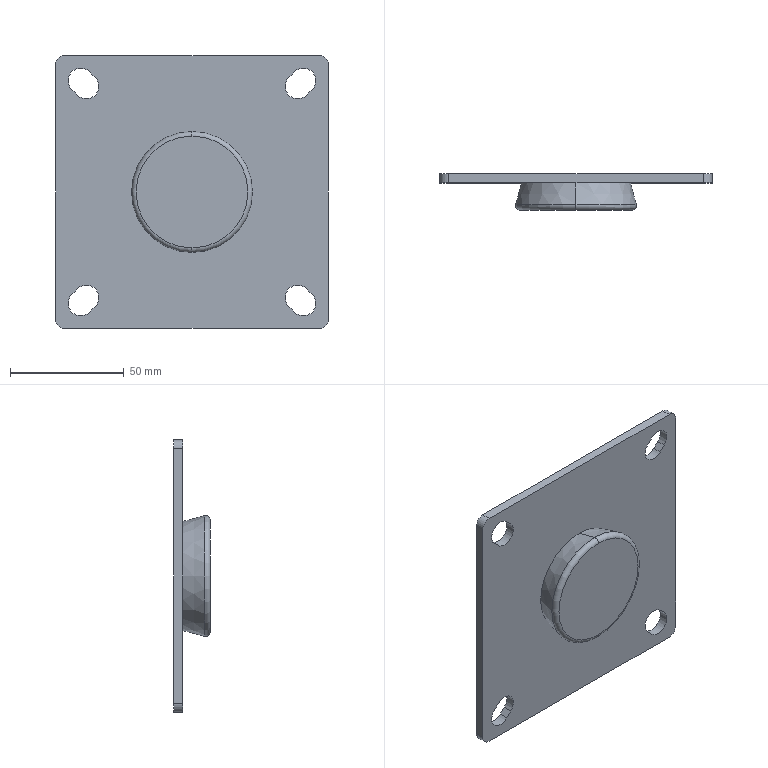Part | STEP file | JAJ-65_plate | 1 solid | 31 faces | box 120 x 16 x 120 mm | volume 79899 mm3 | plane 15 | cylinder 12 | torus 2 | cone 2 | commonest cylinder face diameters 11 x8 8 x4
STEP:
#1=CARTESIAN_POINT('',(0.,-9.482,26.541));
#2=VERTEX_POINT('',#1);
#3=CARTESIAN_POINT('',(0.,-9.482,-26.541));
#4=VERTEX_POINT('',#3);
#5=CARTESIAN_POINT('',(0.,-9.482,0.));
#6=DIRECTION('',(0.,-1.,0.));
#7=DIRECTION('',(0.,0.,-1.));
#8=AXIS2_PLACEMENT_3D('',#5,#6,#7);
#9=CIRCLE('',#8,26.541);
#10=EDGE_CURVE('',#2,#4,#9,.T.);
#11=ORIENTED_EDGE('',*,*,#10,.T.);
#12=CARTESIAN_POINT('',(0.,-12.,-24.609));
#13=VERTEX_POINT('',#12);
#14=CARTESIAN_POINT('',(0.,-10.,-24.609));
#15=DIRECTION('',(-1.,0.,0.));
#16=DIRECTION('',(0.,0.,1.));
#17=AXIS2_PLACEMENT_3D('',#14,#15,#16);
#18=CIRCLE('',#17,2.);
#19=EDGE_CURVE('',#4,#13,#18,.T.);
#20=ORIENTED_EDGE('',*,*,#19,.T.);
#21=CARTESIAN_POINT('',(0.,-12.,24.609));
#22=VERTEX_POINT('',#21);
#23=CARTESIAN_POINT('',(0.,-12.,0.));
#24=DIRECTION('',(0.,-1.,0.));
#25=DIRECTION('',(0.,0.,1.));
#26=AXIS2_PLACEMENT_3D('',#23,#24,#25);
#27=CIRCLE('',#26,24.609);
#28=EDGE_CURVE('',#22,#13,#27,.T.);
#29=ORIENTED_EDGE('',*,*,#28,.F.);
#30=CARTESIAN_POINT('',(0.,-10.,24.609));
#31=DIRECTION('',(1.,0.,0.));
#32=DIRECTION('',(0.,0.,-1.));
#33=AXIS2_PLACEMENT_3D('',#30,#31,#32);
#34=CIRCLE('',#33,2.);
#35=EDGE_CURVE('',#2,#22,#34,.T.);
#36=ORIENTED_EDGE('',*,*,#35,.F.);
#37=EDGE_LOOP('',(#11,#20,#29,#36));
#38=FACE_OUTER_BOUND('',#37,.T.);
#39=CARTESIAN_POINT('',(0.,-10.,0.));
#40=DIRECTION('',(0.,-1.,0.));
#41=DIRECTION('',(0.,0.,1.));
#42=AXIS2_PLACEMENT_3D('',#39,#40,#41);
#43=TOROIDAL_SURFACE('',#42,24.609,2.);
#44=ADVANCED_FACE('',(#38),#43,.T.);
#45=CARTESIAN_POINT('',(0.,0.,24.));
#46=VERTEX_POINT('',#45);
#47=CARTESIAN_POINT('',(0.,0.,-24.));
#48=VERTEX_POINT('',#47);
#49=CARTESIAN_POINT('',(0.,0.,0.));
#50=DIRECTION('',(0.,-1.,0.));
#51=DIRECTION('',(0.,0.,-1.));
#52=AXIS2_PLACEMENT_3D('',#49,#50,#51);
#53=CIRCLE('',#52,24.);
#54=EDGE_CURVE('',#46,#48,#53,.T.);
#55=ORIENTED_EDGE('',*,*,#54,.T.);
#56=CARTESIAN_POINT('',(0.,-9.482,-26.541));
#57=DIRECTION('',(0.,-0.9659,-0.2588));
#58=VECTOR('',#57,1000.);
#59=LINE('',#56,#58);
#60=EDGE_CURVE('',#48,#4,#59,.T.);
#61=ORIENTED_EDGE('',*,*,#60,.T.);
#62=ORIENTED_EDGE('',*,*,#10,.F.);
#63=CARTESIAN_POINT('',(0.,-9.482,26.541));
#64=DIRECTION('',(0.,-0.9659,0.2588));
#65=VECTOR('',#64,1000.);
#66=LINE('',#63,#65);
#67=EDGE_CURVE('',#46,#2,#66,.T.);
#68=ORIENTED_EDGE('',*,*,#67,.F.);
#69=EDGE_LOOP('',(#55,#61,#62,#68));
#70=FACE_OUTER_BOUND('',#69,.T.);
#71=CARTESIAN_POINT('',(0.,-9.482,0.));
#72=DIRECTION('',(0.,-1.,0.));
#73=DIRECTION('',(0.,0.,1.));
#74=AXIS2_PLACEMENT_3D('',#71,#72,#73);
#75=CONICAL_SURFACE('',#74,26.541,0.2618);
#76=ADVANCED_FACE('',(#70),#75,.T.);
#77=CARTESIAN_POINT('',(-60.,0.,-56.));
#78=VERTEX_POINT('',#77);
#79=CARTESIAN_POINT('',(-60.,0.,56.));
#80=VERTEX_POINT('',#79);
#81=CARTESIAN_POINT('',(-60.,0.,-56.));
#82=DIRECTION('',(0.,0.,1.));
#83=VECTOR('',#82,1000.);
#84=LINE('',#81,#83);
#85=EDGE_CURVE('',#78,#80,#84,.T.);
#86=ORIENTED_EDGE('',*,*,#85,.T.);
#87=CARTESIAN_POINT('',(-60.,4.,56.));
#88=VERTEX_POINT('',#87);
#89=CARTESIAN_POINT('',(-60.,0.,56.));
#90=DIRECTION('',(0.,-1.,0.));
#91=VECTOR('',#90,1000.);
#92=LINE('',#89,#91);
#93=EDGE_CURVE('',#88,#80,#92,.T.);
#94=ORIENTED_EDGE('',*,*,#93,.F.);
#95=CARTESIAN_POINT('',(-60.,4.,-56.));
#96=VERTEX_POINT('',#95);
#97=CARTESIAN_POINT('',(-60.,4.,56.));
#98=DIRECTION('',(0.,0.,1.));
#99=VECTOR('',#98,1000.);
#100=LINE('',#97,#99);
#101=EDGE_CURVE('',#96,#88,#100,.T.);
#102=ORIENTED_EDGE('',*,*,#101,.F.);
#103=CARTESIAN_POINT('',(-60.,4.,-56.));
#104=DIRECTION('',(0.,-1.,0.));
#105=VECTOR('',#104,1000.);
#106=LINE('',#103,#105);
#107=EDGE_CURVE('',#96,#78,#106,.T.);
#108=ORIENTED_EDGE('',*,*,#107,.T.);
#109=EDGE_LOOP('',(#86,#94,#102,#108));
#110=FACE_OUTER_BOUND('',#109,.T.);
#111=CARTESIAN_POINT('',(-60.,0.,56.));
#112=DIRECTION('',(-1.,0.,0.));
#113=DIRECTION('',(0.,1.,0.));
#114=AXIS2_PLACEMENT_3D('',#111,#112,#113);
#115=PLANE('',#114);
#116=ADVANCED_FACE('',(#110),#115,.T.);
#117=CARTESIAN_POINT('',(-56.,0.,60.));
#118=VERTEX_POINT('',#117);
#119=CARTESIAN_POINT('',(-56.,0.,56.));
#120=DIRECTION('',(0.,1.,0.));
#121=DIRECTION('',(-1.,0.,0.));
#122=AXIS2_PLACEMENT_3D('',#119,#120,#121);
#123=CIRCLE('',#122,4.);
#124=EDGE_CURVE('',#80,#118,#123,.T.);
#125=ORIENTED_EDGE('',*,*,#124,.T.);
#126=CARTESIAN_POINT('',(-56.,4.,60.));
#127=VERTEX_POINT('',#126);
#128=CARTESIAN_POINT('',(-56.,0.,60.));
#129=DIRECTION('',(0.,-1.,0.));
#130=VECTOR('',#129,1000.);
#131=LINE('',#128,#130);
#132=EDGE_CURVE('',#127,#118,#131,.T.);
#133=ORIENTED_EDGE('',*,*,#132,.F.);
#134=CARTESIAN_POINT('',(-56.,4.,56.));
#135=DIRECTION('',(0.,1.,0.));
#136=DIRECTION('',(0.,0.,1.));
#137=AXIS2_PLACEMENT_3D('',#134,#135,#136);
#138=CIRCLE('',#137,4.);
#139=EDGE_CURVE('',#88,#127,#138,.T.);
#140=ORIENTED_EDGE('',*,*,#139,.F.);
#141=ORIENTED_EDGE('',*,*,#93,.T.);
#142=EDGE_LOOP('',(#125,#133,#140,#141));
#143=FACE_OUTER_BOUND('',#142,.T.);
#144=CARTESIAN_POINT('',(-56.,4.,56.));
#145=DIRECTION('',(0.,-1.,0.));
#146=DIRECTION('',(0.,0.,1.));
#147=AXIS2_PLACEMENT_3D('',#144,#145,#146);
#148=CYLINDRICAL_SURFACE('',#147,4.);
#149=ADVANCED_FACE('',(#143),#148,.T.);
#150=CARTESIAN_POINT('',(56.,0.,60.));
#151=VERTEX_POINT('',#150);
#152=CARTESIAN_POINT('',(-56.,0.,60.));
#153=DIRECTION('',(1.,0.,0.));
#154=VECTOR('',#153,1000.);
#155=LINE('',#152,#154);
#156=EDGE_CURVE('',#118,#151,#155,.T.);
#157=ORIENTED_EDGE('',*,*,#156,.T.);
#158=CARTESIAN_POINT('',(56.,4.,60.));
#159=VERTEX_POINT('',#158);
#160=CARTESIAN_POINT('',(56.,0.,60.));
#161=DIRECTION('',(0.,-1.,0.));
#162=VECTOR('',#161,1000.);
#163=LINE('',#160,#162);
#164=EDGE_CURVE('',#159,#151,#163,.T.);
#165=ORIENTED_EDGE('',*,*,#164,.F.);
#166=CARTESIAN_POINT('',(56.,4.,60.));
#167=DIRECTION('',(1.,0.,0.));
#168=VECTOR('',#167,1000.);
#169=LINE('',#166,#168);
#170=EDGE_CURVE('',#127,#159,#169,.T.);
#171=ORIENTED_EDGE('',*,*,#170,.F.);
#172=ORIENTED_EDGE('',*,*,#132,.T.);
#173=EDGE_LOOP('',(#157,#165,#171,#172));
#174=FACE_OUTER_BOUND('',#173,.T.);
#175=CARTESIAN_POINT('',(56.,0.,60.));
#176=DIRECTION('',(0.,0.,1.));
#177=DIRECTION('',(0.,1.,0.));
#178=AXIS2_PLACEMENT_3D('',#175,#176,#177);
#179=PLANE('',#178);
#180=ADVANCED_FACE('',(#174),#179,.T.);
#181=CARTESIAN_POINT('',(60.,0.,56.));
#182=VERTEX_POINT('',#181);
#183=CARTESIAN_POINT('',(56.,0.,56.));
#184=DIRECTION('',(0.,1.,0.));
#185=DIRECTION('',(0.,0.,1.));
#186=AXIS2_PLACEMENT_3D('',#183,#184,#185);
#187=CIRCLE('',#186,4.);
#188=EDGE_CURVE('',#151,#182,#187,.T.);
#189=ORIENTED_EDGE('',*,*,#188,.T.);
#190=CARTESIAN_POINT('',(60.,4.,56.));
#191=VERTEX_POINT('',#190);
#192=CARTESIAN_POINT('',(60.,0.,56.));
#193=DIRECTION('',(0.,-1.,0.));
#194=VECTOR('',#193,1000.);
#195=LINE('',#192,#194);
#196=EDGE_CURVE('',#191,#182,#195,.T.);
#197=ORIENTED_EDGE('',*,*,#196,.F.);
#198=CARTESIAN_POINT('',(56.,4.,56.));
#199=DIRECTION('',(0.,1.,0.));
#200=DIRECTION('',(1.,0.,0.));
#201=AXIS2_PLACEMENT_3D('',#198,#199,#200);
#202=CIRCLE('',#201,4.);
#203=EDGE_CURVE('',#159,#191,#202,.T.);
#204=ORIENTED_EDGE('',*,*,#203,.F.);
#205=ORIENTED_EDGE('',*,*,#164,.T.);
#206=EDGE_LOOP('',(#189,#197,#204,#205));
#207=FACE_OUTER_BOUND('',#206,.T.);
#208=CARTESIAN_POINT('',(56.,4.,56.));
#209=DIRECTION('',(0.,-1.,0.));
#210=DIRECTION('',(1.,0.,0.));
#211=AXIS2_PLACEMENT_3D('',#208,#209,#210);
#212=CYLINDRICAL_SURFACE('',#211,4.);
#213=ADVANCED_FACE('',(#207),#212,.T.);
#214=CARTESIAN_POINT('',(60.,0.,-56.));
#215=VERTEX_POINT('',#214);
#216=CARTESIAN_POINT('',(60.,0.,56.));
#217=DIRECTION('',(0.,0.,-1.));
#218=VECTOR('',#217,1000.);
#219=LINE('',#216,#218);
#220=EDGE_CURVE('',#182,#215,#219,.T.);
#221=ORIENTED_EDGE('',*,*,#220,.T.);
#222=CARTESIAN_POINT('',(60.,4.,-56.));
#223=VERTEX_POINT('',#222);
#224=CARTESIAN_POINT('',(60.,0.,-56.));
#225=DIRECTION('',(0.,-1.,0.));
#226=VECTOR('',#225,1000.);
#227=LINE('',#224,#226);
#228=EDGE_CURVE('',#223,#215,#227,.T.);
#229=ORIENTED_EDGE('',*,*,#228,.F.);
#230=CARTESIAN_POINT('',(60.,4.,-56.));
#231=DIRECTION('',(0.,0.,-1.));
#232=VECTOR('',#231,1000.);
#233=LINE('',#230,#232);
#234=EDGE_CURVE('',#191,#223,#233,.T.);
#235=ORIENTED_EDGE('',*,*,#234,.F.);
#236=ORIENTED_EDGE('',*,*,#196,.T.);
#237=EDGE_LOOP('',(#221,#229,#235,#236));
#238=FACE_OUTER_BOUND('',#237,.T.);
#239=CARTESIAN_POINT('',(60.,0.,-56.));
#240=DIRECTION('',(1.,0.,0.));
#241=DIRECTION('',(0.,1.,0.));
#242=AXIS2_PLACEMENT_3D('',#239,#240,#241);
#243=PLANE('',#242);
#244=ADVANCED_FACE('',(#238),#243,.T.);
#245=CARTESIAN_POINT('',(56.,0.,-60.));
#246=VERTEX_POINT('',#245);
#247=CARTESIAN_POINT('',(56.,0.,-56.));
#248=DIRECTION('',(0.,1.,0.));
#249=DIRECTION('',(1.,0.,0.));
#250=AXIS2_PLACEMENT_3D('',#247,#248,#249);
#251=CIRCLE('',#250,4.);
#252=EDGE_CURVE('',#215,#246,#251,.T.);
#253=ORIENTED_EDGE('',*,*,#252,.T.);
#254=CARTESIAN_POINT('',(56.,4.,-60.));
#255=VERTEX_POINT('',#254);
#256=CARTESIAN_POINT('',(56.,0.,-60.));
#257=DIRECTION('',(0.,-1.,0.));
#258=VECTOR('',#257,1000.);
#259=LINE('',#256,#258);
#260=EDGE_CURVE('',#255,#246,#259,.T.);
#261=ORIENTED_EDGE('',*,*,#260,.F.);
#262=CARTESIAN_POINT('',(56.,4.,-56.));
#263=DIRECTION('',(0.,1.,0.));
#264=DIRECTION('',(0.,0.,-1.));
#265=AXIS2_PLACEMENT_3D('',#262,#263,#264);
#266=CIRCLE('',#265,4.);
#267=EDGE_CURVE('',#223,#255,#266,.T.);
#268=ORIENTED_EDGE('',*,*,#267,.F.);
#269=ORIENTED_EDGE('',*,*,#228,.T.);
#270=EDGE_LOOP('',(#253,#261,#268,#269));
#271=FACE_OUTER_BOUND('',#270,.T.);
#272=CARTESIAN_POINT('',(56.,4.,-56.));
#273=DIRECTION('',(0.,-1.,0.));
#274=DIRECTION('',(0.,0.,-1.));
#275=AXIS2_PLACEMENT_3D('',#272,#273,#274);
#276=CYLINDRICAL_SURFACE('',#275,4.);
#277=ADVANCED_FACE('',(#271),#276,.T.);
#278=CARTESIAN_POINT('',(-56.,0.,-60.));
#279=VERTEX_POINT('',#278);
#280=CARTESIAN_POINT('',(56.,0.,-60.));
#281=DIRECTION('',(-1.,0.,0.));
#282=VECTOR('',#281,1000.);
#283=LINE('',#280,#282);
#284=EDGE_CURVE('',#246,#279,#283,.T.);
#285=ORIENTED_EDGE('',*,*,#284,.T.);
#286=CARTESIAN_POINT('',(-56.,4.,-60.));
#287=VERTEX_POINT('',#286);
#288=CARTESIAN_POINT('',(-56.,0.,-60.));
#289=DIRECTION('',(0.,-1.,0.));
#290=VECTOR('',#289,1000.);
#291=LINE('',#288,#290);
#292=EDGE_CURVE('',#287,#279,#291,.T.);
#293=ORIENTED_EDGE('',*,*,#292,.F.);
#294=CARTESIAN_POINT('',(-56.,4.,-60.));
#295=DIRECTION('',(-1.,0.,0.));
#296=VECTOR('',#295,1000.);
#297=LINE('',#294,#296);
#298=EDGE_CURVE('',#255,#287,#297,.T.);
#299=ORIENTED_EDGE('',*,*,#298,.F.);
#300=ORIENTED_EDGE('',*,*,#260,.T.);
#301=EDGE_LOOP('',(#285,#293,#299,#300));
#302=FACE_OUTER_BOUND('',#301,.T.);
#303=CARTESIAN_POINT('',(-56.,0.,-60.));
#304=DIRECTION('',(0.,0.,-1.));
#305=DIRECTION('',(0.,1.,0.));
#306=AXIS2_PLACEMENT_3D('',#303,#304,#305);
#307=PLANE('',#306);
#308=ADVANCED_FACE('',(#302),#307,.T.);
#309=CARTESIAN_POINT('',(45.111,0.,-52.889));
#310=VERTEX_POINT('',#309);
#311=CARTESIAN_POINT('',(42.611,0.,-50.389));
#312=VERTEX_POINT('',#311);
#313=CARTESIAN_POINT('',(42.611,0.,-50.389));
#314=DIRECTION('',(-0.7071,0.,0.7071));
#315=VECTOR('',#314,1000.);
#316=LINE('',#313,#315);
#317=EDGE_CURVE('',#310,#312,#316,.T.);
#318=ORIENTED_EDGE('',*,*,#317,.F.);
#319=CARTESIAN_POINT('',(45.111,4.,-52.889));
#320=VERTEX_POINT('',#319);
#321=CARTESIAN_POINT('',(45.111,0.,-52.889));
#322=DIRECTION('',(0.,-1.,0.));
#323=VECTOR('',#322,1000.);
#324=LINE('',#321,#323);
#325=EDGE_CURVE('',#320,#310,#324,.T.);
#326=ORIENTED_EDGE('',*,*,#325,.F.);
#327=CARTESIAN_POINT('',(42.611,4.,-50.389));
#328=VERTEX_POINT('',#327);
#329=CARTESIAN_POINT('',(45.111,4.,-52.889));
#330=DIRECTION('',(-0.7071,0.,0.7071));
#331=VECTOR('',#330,1000.);
#332=LINE('',#329,#331);
#333=EDGE_CURVE('',#320,#328,#332,.T.);
#334=ORIENTED_EDGE('',*,*,#333,.T.);
#335=CARTESIAN_POINT('',(42.611,4.,-50.389));
#336=DIRECTION('',(0.,-1.,0.));
#337=VECTOR('',#336,1000.);
#338=LINE('',#335,#337);
#339=EDGE_CURVE('',#328,#312,#338,.T.);
#340=ORIENTED_EDGE('',*,*,#339,.T.);
#341=EDGE_LOOP('',(#318,#326,#334,#340));
#342=FACE_OUTER_BOUND('',#341,.T.);
#343=CARTESIAN_POINT('',(42.611,0.,-50.389));
#344=DIRECTION('',(0.7071,0.,0.7071));
#345=DIRECTION('',(0.7071,0.,-0.7071));
#346=AXIS2_PLACEMENT_3D('',#343,#344,#345);
#347=PLANE('',#346);
#348=ADVANCED_FACE('',(#342),#347,.T.);
#349=CARTESIAN_POINT('',(52.889,0.,-45.111));
#350=VERTEX_POINT('',#349);
#351=CARTESIAN_POINT('',(49.,0.,-49.));
#352=DIRECTION('',(0.,1.,0.));
#353=DIRECTION('',(-0.7071,0.,-0.7071));
#354=AXIS2_PLACEMENT_3D('',#351,#352,#353);
#355=CIRCLE('',#354,5.5);
#356=EDGE_CURVE('',#350,#310,#355,.T.);
#357=ORIENTED_EDGE('',*,*,#356,.F.);
#358=CARTESIAN_POINT('',(52.889,4.,-45.111));
#359=VERTEX_POINT('',#358);
#360=CARTESIAN_POINT('',(52.889,0.,-45.111));
#361=DIRECTION('',(0.,-1.,0.));
#362=VECTOR('',#361,1000.);
#363=LINE('',#360,#362);
#364=EDGE_CURVE('',#359,#350,#363,.T.);
#365=ORIENTED_EDGE('',*,*,#364,.F.);
#366=CARTESIAN_POINT('',(49.,4.,-49.));
#367=DIRECTION('',(0.,1.,0.));
#368=DIRECTION('',(0.7071,0.,0.7071));
#369=AXIS2_PLACEMENT_3D('',#366,#367,#368);
#370=CIRCLE('',#369,5.5);
#371=EDGE_CURVE('',#359,#320,#370,.T.);
#372=ORIENTED_EDGE('',*,*,#371,.T.);
#373=ORIENTED_EDGE('',*,*,#325,.T.);
#374=EDGE_LOOP('',(#357,#365,#372,#373));
#375=FACE_OUTER_BOUND('',#374,.T.);
#376=CARTESIAN_POINT('',(49.,4.,-49.));
#377=DIRECTION('',(0.,-1.,0.));
#378=DIRECTION('',(-0.7071,0.,-0.7071));
#379=AXIS2_PLACEMENT_3D('',#376,#377,#378);
#380=CYLINDRICAL_SURFACE('',#379,5.5);
#381=ADVANCED_FACE('',(#375),#380,.F.);
#382=CARTESIAN_POINT('',(50.389,0.,-42.611));
#383=VERTEX_POINT('',#382);
#384=CARTESIAN_POINT('',(52.889,0.,-45.111));
#385=DIRECTION('',(0.7071,0.,-0.7071));
#386=VECTOR('',#385,1000.);
#387=LINE('',#384,#386);
#388=EDGE_CURVE('',#383,#350,#387,.T.);
#389=ORIENTED_EDGE('',*,*,#388,.F.);
#390=CARTESIAN_POINT('',(50.389,4.,-42.611));
#391=VERTEX_POINT('',#390);
#392=CARTESIAN_POINT('',(50.389,0.,-42.611));
#393=DIRECTION('',(0.,-1.,0.));
#394=VECTOR('',#393,1000.);
#395=LINE('',#392,#394);
#396=EDGE_CURVE('',#391,#383,#395,.T.);
#397=ORIENTED_EDGE('',*,*,#396,.F.);
#398=CARTESIAN_POINT('',(50.389,4.,-42.611));
#399=DIRECTION('',(0.7071,0.,-0.7071));
#400=VECTOR('',#399,1000.);
#401=LINE('',#398,#400);
#402=EDGE_CURVE('',#391,#359,#401,.T.);
#403=ORIENTED_EDGE('',*,*,#402,.T.);
#404=ORIENTED_EDGE('',*,*,#364,.T.);
#405=EDGE_LOOP('',(#389,#397,#403,#404));
#406=FACE_OUTER_BOUND('',#405,.T.);
#407=CARTESIAN_POINT('',(52.889,0.,-45.111));
#408=DIRECTION('',(-0.7071,0.,-0.7071));
#409=DIRECTION('',(-0.7071,0.,0.7071));
#410=AXIS2_PLACEMENT_3D('',#407,#408,#409);
#411=PLANE('',#410);
#412=ADVANCED_FACE('',(#406),#411,.T.);
#413=CARTESIAN_POINT('',(52.889,0.,45.111));
#414=VERTEX_POINT('',#413);
#415=CARTESIAN_POINT('',(50.389,0.,42.611));
#416=VERTEX_POINT('',#415);
#417=CARTESIAN_POINT('',(50.389,0.,42.611));
#418=DIRECTION('',(-0.7071,0.,-0.7071));
#419=VECTOR('',#418,1000.);
#420=LINE('',#417,#419);
#421=EDGE_CURVE('',#414,#416,#420,.T.);
#422=ORIENTED_EDGE('',*,*,#421,.F.);
#423=CARTESIAN_POINT('',(52.889,4.,45.111));
#424=VERTEX_POINT('',#423);
#425=CARTESIAN_POINT('',(52.889,0.,45.111));
#426=DIRECTION('',(0.,-1.,0.));
#427=VECTOR('',#426,1000.);
#428=LINE('',#425,#427);
#429=EDGE_CURVE('',#424,#414,#428,.T.);
#430=ORIENTED_EDGE('',*,*,#429,.F.);
#431=CARTESIAN_POINT('',(50.389,4.,42.611));
#432=VERTEX_POINT('',#431);
#433=CARTESIAN_POINT('',(52.889,4.,45.111));
#434=DIRECTION('',(-0.7071,0.,-0.7071));
#435=VECTOR('',#434,1000.);
#436=LINE('',#433,#435);
#437=EDGE_CURVE('',#424,#432,#436,.T.);
#438=ORIENTED_EDGE('',*,*,#437,.T.);
#439=CARTESIAN_POINT('',(50.389,4.,42.611));
#440=DIRECTION('',(0.,-1.,0.));
#441=VECTOR('',#440,1000.);
#442=LINE('',#439,#441);
#443=EDGE_CURVE('',#432,#416,#442,.T.);
#444=ORIENTED_EDGE('',*,*,#443,.T.);
#445=EDGE_LOOP('',(#422,#430,#438,#444));
#446=FACE_OUTER_BOUND('',#445,.T.);
#447=CARTESIAN_POINT('',(50.389,0.,42.611));
#448=DIRECTION('',(-0.7071,0.,0.7071));
#449=DIRECTION('',(0.7071,0.,0.7071));
#450=AXIS2_PLACEMENT_3D('',#447,#448,#449);
#451=PLANE('',#450);
#452=ADVANCED_FACE('',(#446),#451,.T.);
#453=CARTESIAN_POINT('',(45.111,0.,52.889));
#454=VERTEX_POINT('',#453);
#455=CARTESIAN_POINT('',(49.,0.,49.));
#456=DIRECTION('',(0.,1.,0.));
#457=DIRECTION('',(0.7071,0.,-0.7071));
#458=AXIS2_PLACEMENT_3D('',#455,#456,#457);
#459=CIRCLE('',#458,5.5);
#460=EDGE_CURVE('',#454,#414,#459,.T.);
#461=ORIENTED_EDGE('',*,*,#460,.F.);
#462=CARTESIAN_POINT('',(45.111,4.,52.889));
#463=VERTEX_POINT('',#462);
#464=CARTESIAN_POINT('',(45.111,0.,52.889));
#465=DIRECTION('',(0.,-1.,0.));
#466=VECTOR('',#465,1000.);
#467=LINE('',#464,#466);
#468=EDGE_CURVE('',#463,#454,#467,.T.);
#469=ORIENTED_EDGE('',*,*,#468,.F.);
#470=CARTESIAN_POINT('',(49.,4.,49.));
#471=DIRECTION('',(0.,1.,0.));
#472=DIRECTION('',(-0.7071,0.,0.7071));
#473=AXIS2_PLACEMENT_3D('',#470,#471,#472);
#474=CIRCLE('',#473,5.5);
#475=EDGE_CURVE('',#463,#424,#474,.T.);
#476=ORIENTED_EDGE('',*,*,#475,.T.);
#477=ORIENTED_EDGE('',*,*,#429,.T.);
#478=EDGE_LOOP('',(#461,#469,#476,#477));
#479=FACE_OUTER_BOUND('',#478,.T.);
#480=CARTESIAN_POINT('',(49.,4.,49.));
#481=DIRECTION('',(0.,-1.,0.));
#482=DIRECTION('',(0.7071,0.,-0.7071));
#483=AXIS2_PLACEMENT_3D('',#480,#481,#482);
#484=CYLINDRICAL_SURFACE('',#483,5.5);
#485=ADVANCED_FACE('',(#479),#484,.F.);
#486=CARTESIAN_POINT('',(42.611,0.,50.389));
#487=VERTEX_POINT('',#486);
#488=CARTESIAN_POINT('',(45.111,0.,52.889));
#489=DIRECTION('',(0.7071,0.,0.7071));
#490=VECTOR('',#489,1000.);
#491=LINE('',#488,#490);
#492=EDGE_CURVE('',#487,#454,#491,.T.);
#493=ORIENTED_EDGE('',*,*,#492,.F.);
#494=CARTESIAN_POINT('',(42.611,4.,50.389));
#495=VERTEX_POINT('',#494);
#496=CARTESIAN_POINT('',(42.611,0.,50.389));
#497=DIRECTION('',(0.,-1.,0.));
#498=VECTOR('',#497,1000.);
#499=LINE('',#496,#498);
#500=EDGE_CURVE('',#495,#487,#499,.T.);
#501=ORIENTED_EDGE('',*,*,#500,.F.);
#502=CARTESIAN_POINT('',(42.611,4.,50.389));
#503=DIRECTION('',(0.7071,0.,0.7071));
#504=VECTOR('',#503,1000.);
#505=LINE('',#502,#504);
#506=EDGE_CURVE('',#495,#463,#505,.T.);
#507=ORIENTED_EDGE('',*,*,#506,.T.);
#508=ORIENTED_EDGE('',*,*,#468,.T.);
#509=EDGE_LOOP('',(#493,#501,#507,#508));
#510=FACE_OUTER_BOUND('',#509,.T.);
#511=CARTESIAN_POINT('',(45.111,0.,52.889));
#512=DIRECTION('',(0.7071,0.,-0.7071));
#513=DIRECTION('',(-0.7071,0.,-0.7071));
#514=AXIS2_PLACEMENT_3D('',#511,#512,#513);
#515=PLANE('',#514);
#516=ADVANCED_FACE('',(#510),#515,.T.);
#517=CARTESIAN_POINT('',(-42.611,0.,-50.389));
#518=VERTEX_POINT('',#517);
#519=CARTESIAN_POINT('',(-45.111,0.,-52.889));
#520=VERTEX_POINT('',#519);
#521=CARTESIAN_POINT('',(-45.111,0.,-52.889));
#522=DIRECTION('',(-0.7071,0.,-0.7071));
#523=VECTOR('',#522,1000.);
#524=LINE('',#521,#523);
#525=EDGE_CURVE('',#518,#520,#524,.T.);
#526=ORIENTED_EDGE('',*,*,#525,.F.);
#527=CARTESIAN_POINT('',(-42.611,4.,-50.389));
#528=VERTEX_POINT('',#527);
#529=CARTESIAN_POINT('',(-42.611,0.,-50.389));
#530=DIRECTION('',(0.,-1.,0.));
#531=VECTOR('',#530,1000.);
#532=LINE('',#529,#531);
#533=EDGE_CURVE('',#528,#518,#532,.T.);
#534=ORIENTED_EDGE('',*,*,#533,.F.);
#535=CARTESIAN_POINT('',(-45.111,4.,-52.889));
#536=VERTEX_POINT('',#535);
#537=CARTESIAN_POINT('',(-42.611,4.,-50.389));
#538=DIRECTION('',(-0.7071,0.,-0.7071));
#539=VECTOR('',#538,1000.);
#540=LINE('',#537,#539);
#541=EDGE_CURVE('',#528,#536,#540,.T.);
#542=ORIENTED_EDGE('',*,*,#541,.T.);
#543=CARTESIAN_POINT('',(-45.111,4.,-52.889));
#544=DIRECTION('',(0.,-1.,0.));
#545=VECTOR('',#544,1000.);
#546=LINE('',#543,#545);
#547=EDGE_CURVE('',#536,#520,#546,.T.);
#548=ORIENTED_EDGE('',*,*,#547,.T.);
#549=EDGE_LOOP('',(#526,#534,#542,#548));
#550=FACE_OUTER_BOUND('',#549,.T.);
#551=CARTESIAN_POINT('',(-45.111,0.,-52.889));
#552=DIRECTION('',(-0.7071,0.,0.7071));
#553=DIRECTION('',(0.7071,0.,0.7071));
#554=AXIS2_PLACEMENT_3D('',#551,#552,#553);
#555=PLANE('',#554);
#556=ADVANCED_FACE('',(#550),#555,.T.);
#557=CARTESIAN_POINT('',(-50.389,0.,-42.611));
#558=VERTEX_POINT('',#557);
#559=CARTESIAN_POINT('',(-46.5,0.,-46.5));
#560=DIRECTION('',(0.,1.,0.));
#561=DIRECTION('',(0.7071,0.,-0.7071));
#562=AXIS2_PLACEMENT_3D('',#559,#560,#561);
#563=CIRCLE('',#562,5.5);
#564=EDGE_CURVE('',#558,#518,#563,.T.);
#565=ORIENTED_EDGE('',*,*,#564,.F.);
#566=CARTESIAN_POINT('',(-50.389,4.,-42.611));
#567=VERTEX_POINT('',#566);
#568=CARTESIAN_POINT('',(-50.389,0.,-42.611));
#569=DIRECTION('',(0.,-1.,0.));
#570=VECTOR('',#569,1000.);
#571=LINE('',#568,#570);
#572=EDGE_CURVE('',#567,#558,#571,.T.);
#573=ORIENTED_EDGE('',*,*,#572,.F.);
#574=CARTESIAN_POINT('',(-46.5,4.,-46.5));
#575=DIRECTION('',(0.,1.,0.));
#576=DIRECTION('',(-0.7071,0.,0.7071));
#577=AXIS2_PLACEMENT_3D('',#574,#575,#576);
#578=CIRCLE('',#577,5.5);
#579=EDGE_CURVE('',#567,#528,#578,.T.);
#580=ORIENTED_EDGE('',*,*,#579,.T.);
#581=ORIENTED_EDGE('',*,*,#533,.T.);
#582=EDGE_LOOP('',(#565,#573,#580,#581));
#583=FACE_OUTER_BOUND('',#582,.T.);
#584=CARTESIAN_POINT('',(-46.5,4.,-46.5));
#585=DIRECTION('',(0.,-1.,0.));
#586=DIRECTION('',(0.7071,0.,-0.7071));
#587=AXIS2_PLACEMENT_3D('',#584,#585,#586);
#588=CYLINDRICAL_SURFACE('',#587,5.5);
#589=ADVANCED_FACE('',(#583),#588,.F.);
#590=CARTESIAN_POINT('',(-52.889,0.,-45.111));
#591=VERTEX_POINT('',#590);
#592=CARTESIAN_POINT('',(-50.389,0.,-42.611));
#593=DIRECTION('',(0.7071,0.,0.7071));
#594=VECTOR('',#593,1000.);
#595=LINE('',#592,#594);
#596=EDGE_CURVE('',#591,#558,#595,.T.);
#597=ORIENTED_EDGE('',*,*,#596,.F.);
#598=CARTESIAN_POINT('',(-52.889,4.,-45.111));
#599=VERTEX_POINT('',#598);
#600=CARTESIAN_POINT('',(-52.889,0.,-45.111));
#601=DIRECTION('',(0.,-1.,0.));
#602=VECTOR('',#601,1000.);
#603=LINE('',#600,#602);
#604=EDGE_CURVE('',#599,#591,#603,.T.);
#605=ORIENTED_EDGE('',*,*,#604,.F.);
#606=CARTESIAN_POINT('',(-52.889,4.,-45.111));
#607=DIRECTION('',(0.7071,0.,0.7071));
#608=VECTOR('',#607,1000.);
#609=LINE('',#606,#608);
#610=EDGE_CURVE('',#599,#567,#609,.T.);
#611=ORIENTED_EDGE('',*,*,#610,.T.);
#612=ORIENTED_EDGE('',*,*,#572,.T.);
#613=EDGE_LOOP('',(#597,#605,#611,#612));
#614=FACE_OUTER_BOUND('',#613,.T.);
#615=CARTESIAN_POINT('',(-50.389,0.,-42.611));
#616=DIRECTION('',(0.7071,0.,-0.7071));
#617=DIRECTION('',(-0.7071,0.,-0.7071));
#618=AXIS2_PLACEMENT_3D('',#615,#616,#617);
#619=PLANE('',#618);
#620=ADVANCED_FACE('',(#614),#619,.T.);
#621=CARTESIAN_POINT('',(-50.389,0.,42.611));
#622=VERTEX_POINT('',#621);
#623=CARTESIAN_POINT('',(-52.889,0.,45.111));
#624=VERTEX_POINT('',#623);
#625=CARTESIAN_POINT('',(-52.889,0.,45.111));
#626=DIRECTION('',(-0.7071,0.,0.7071));
#627=VECTOR('',#626,1000.);
#628=LINE('',#625,#627);
#629=EDGE_CURVE('',#622,#624,#628,.T.);
#630=ORIENTED_EDGE('',*,*,#629,.F.);
#631=CARTESIAN_POINT('',(-50.389,4.,42.611));
#632=VERTEX_POINT('',#631);
#633=CARTESIAN_POINT('',(-50.389,0.,42.611));
#634=DIRECTION('',(0.,-1.,0.));
#635=VECTOR('',#634,1000.);
#636=LINE('',#633,#635);
#637=EDGE_CURVE('',#632,#622,#636,.T.);
#638=ORIENTED_EDGE('',*,*,#637,.F.);
#639=CARTESIAN_POINT('',(-52.889,4.,45.111));
#640=VERTEX_POINT('',#639);
#641=CARTESIAN_POINT('',(-50.389,4.,42.611));
#642=DIRECTION('',(-0.7071,0.,0.7071));
#643=VECTOR('',#642,1000.);
#644=LINE('',#641,#643);
#645=EDGE_CURVE('',#632,#640,#644,.T.);
#646=ORIENTED_EDGE('',*,*,#645,.T.);
#647=CARTESIAN_POINT('',(-52.889,4.,45.111));
#648=DIRECTION('',(0.,-1.,0.));
#649=VECTOR('',#648,1000.);
#650=LINE('',#647,#649);
#651=EDGE_CURVE('',#640,#624,#650,.T.);
#652=ORIENTED_EDGE('',*,*,#651,.T.);
#653=EDGE_LOOP('',(#630,#638,#646,#652));
#654=FACE_OUTER_BOUND('',#653,.T.);
#655=CARTESIAN_POINT('',(-52.889,0.,45.111));
#656=DIRECTION('',(0.7071,0.,0.7071));
#657=DIRECTION('',(0.7071,0.,-0.7071));
#658=AXIS2_PLACEMENT_3D('',#655,#656,#657);
#659=PLANE('',#658);
#660=ADVANCED_FACE('',(#654),#659,.T.);
#661=CARTESIAN_POINT('',(-42.611,0.,50.389));
#662=VERTEX_POINT('',#661);
#663=CARTESIAN_POINT('',(-46.5,0.,46.5));
#664=DIRECTION('',(0.,1.,0.));
#665=DIRECTION('',(-0.7071,0.,-0.7071));
#666=AXIS2_PLACEMENT_3D('',#663,#664,#665);
#667=CIRCLE('',#666,5.5);
#668=EDGE_CURVE('',#662,#622,#667,.T.);
#669=ORIENTED_EDGE('',*,*,#668,.F.);
#670=CARTESIAN_POINT('',(-42.611,4.,50.389));
#671=VERTEX_POINT('',#670);
#672=CARTESIAN_POINT('',(-42.611,0.,50.389));
#673=DIRECTION('',(0.,-1.,0.));
#674=VECTOR('',#673,1000.);
#675=LINE('',#672,#674);
#676=EDGE_CURVE('',#671,#662,#675,.T.);
#677=ORIENTED_EDGE('',*,*,#676,.F.);
#678=CARTESIAN_POINT('',(-46.5,4.,46.5));
#679=DIRECTION('',(0.,1.,0.));
#680=DIRECTION('',(0.7071,0.,0.7071));
#681=AXIS2_PLACEMENT_3D('',#678,#679,#680);
#682=CIRCLE('',#681,5.5);
#683=EDGE_CURVE('',#671,#632,#682,.T.);
#684=ORIENTED_EDGE('',*,*,#683,.T.);
#685=ORIENTED_EDGE('',*,*,#637,.T.);
#686=EDGE_LOOP('',(#669,#677,#684,#685));
#687=FACE_OUTER_BOUND('',#686,.T.);
#688=CARTESIAN_POINT('',(-46.5,4.,46.5));
#689=DIRECTION('',(0.,-1.,0.));
#690=DIRECTION('',(-0.7071,0.,-0.7071));
#691=AXIS2_PLACEMENT_3D('',#688,#689,#690);
#692=CYLINDRICAL_SURFACE('',#691,5.5);
#693=ADVANCED_FACE('',(#687),#692,.F.);
#694=CARTESIAN_POINT('',(-45.111,0.,52.889));
#695=VERTEX_POINT('',#694);
#696=CARTESIAN_POINT('',(-42.611,0.,50.389));
#697=DIRECTION('',(0.7071,0.,-0.7071));
#698=VECTOR('',#697,1000.);
#699=LINE('',#696,#698);
#700=EDGE_CURVE('',#695,#662,#699,.T.);
#701=ORIENTED_EDGE('',*,*,#700,.F.);
#702=CARTESIAN_POINT('',(-45.111,4.,52.889));
#703=VERTEX_POINT('',#702);
#704=CARTESIAN_POINT('',(-45.111,0.,52.889));
#705=DIRECTION('',(0.,-1.,0.));
#706=VECTOR('',#705,1000.);
#707=LINE('',#704,#706);
#708=EDGE_CURVE('',#703,#695,#707,.T.);
#709=ORIENTED_EDGE('',*,*,#708,.F.);
#710=CARTESIAN_POINT('',(-45.111,4.,52.889));
#711=DIRECTION('',(0.7071,0.,-0.7071));
#712=VECTOR('',#711,1000.);
#713=LINE('',#710,#712);
#714=EDGE_CURVE('',#703,#671,#713,.T.);
#715=ORIENTED_EDGE('',*,*,#714,.T.);
#716=ORIENTED_EDGE('',*,*,#676,.T.);
#717=EDGE_LOOP('',(#701,#709,#715,#716));
#718=FACE_OUTER_BOUND('',#717,.T.);
#719=CARTESIAN_POINT('',(-42.611,0.,50.389));
#720=DIRECTION('',(-0.7071,0.,-0.7071));
#721=DIRECTION('',(-0.7071,0.,0.7071));
#722=AXIS2_PLACEMENT_3D('',#719,#720,#721);
#723=PLANE('',#722);
#724=ADVANCED_FACE('',(#718),#723,.T.);
#725=CARTESIAN_POINT('',(46.5,0.,-46.5));
#726=DIRECTION('',(0.,1.,0.));
#727=DIRECTION('',(0.7071,0.,0.7071));
#728=AXIS2_PLACEMENT_3D('',#725,#726,#727);
#729=CIRCLE('',#728,5.5);
#730=EDGE_CURVE('',#312,#383,#729,.T.);
#731=ORIENTED_EDGE('',*,*,#730,.F.);
#732=ORIENTED_EDGE('',*,*,#339,.F.);
#733=CARTESIAN_POINT('',(46.5,4.,-46.5));
#734=DIRECTION('',(0.,1.,0.));
#735=DIRECTION('',(-0.7071,0.,-0.7071));
#736=AXIS2_PLACEMENT_3D('',#733,#734,#735);
#737=CIRCLE('',#736,5.5);
#738=EDGE_CURVE('',#328,#391,#737,.T.);
#739=ORIENTED_EDGE('',*,*,#738,.T.);
#740=ORIENTED_EDGE('',*,*,#396,.T.);
#741=EDGE_LOOP('',(#731,#732,#739,#740));
#742=FACE_OUTER_BOUND('',#741,.T.);
#743=CARTESIAN_POINT('',(46.5,4.,-46.5));
#744=DIRECTION('',(0.,-1.,0.));
#745=DIRECTION('',(0.7071,0.,0.7071));
#746=AXIS2_PLACEMENT_3D('',#743,#744,#745);
#747=CYLINDRICAL_SURFACE('',#746,5.5);
#748=ADVANCED_FACE('',(#742),#747,.F.);
#749=CARTESIAN_POINT('',(46.5,0.,46.5));
#750=DIRECTION('',(0.,1.,0.));
#751=DIRECTION('',(-0.7071,0.,0.7071));
#752=AXIS2_PLACEMENT_3D('',#749,#750,#751);
#753=CIRCLE('',#752,5.5);
#754=EDGE_CURVE('',#416,#487,#753,.T.);
#755=ORIENTED_EDGE('',*,*,#754,.F.);
#756=ORIENTED_EDGE('',*,*,#443,.F.);
#757=CARTESIAN_POINT('',(46.5,4.,46.5));
#758=DIRECTION('',(0.,1.,0.));
#759=DIRECTION('',(0.7071,0.,-0.7071));
#760=AXIS2_PLACEMENT_3D('',#757,#758,#759);
#761=CIRCLE('',#760,5.5);
#762=EDGE_CURVE('',#432,#495,#761,.T.);
#763=ORIENTED_EDGE('',*,*,#762,.T.);
#764=ORIENTED_EDGE('',*,*,#500,.T.);
#765=EDGE_LOOP('',(#755,#756,#763,#764));
#766=FACE_OUTER_BOUND('',#765,.T.);
#767=CARTESIAN_POINT('',(46.5,4.,46.5));
#768=DIRECTION('',(0.,-1.,0.));
#769=DIRECTION('',(-0.7071,0.,0.7071));
#770=AXIS2_PLACEMENT_3D('',#767,#768,#769);
#771=CYLINDRICAL_SURFACE('',#770,5.5);
#772=ADVANCED_FACE('',(#766),#771,.F.);
#773=CARTESIAN_POINT('',(-49.,0.,-49.));
#774=DIRECTION('',(0.,1.,0.));
#775=DIRECTION('',(-0.7071,0.,0.7071));
#776=AXIS2_PLACEMENT_3D('',#773,#774,#775);
#777=CIRCLE('',#776,5.5);
#778=EDGE_CURVE('',#520,#591,#777,.T.);
#779=ORIENTED_EDGE('',*,*,#778,.F.);
#780=ORIENTED_EDGE('',*,*,#547,.F.);
#781=CARTESIAN_POINT('',(-49.,4.,-49.));
#782=DIRECTION('',(0.,1.,0.));
#783=DIRECTION('',(0.7071,0.,-0.7071));
#784=AXIS2_PLACEMENT_3D('',#781,#782,#783);
#785=CIRCLE('',#784,5.5);
#786=EDGE_CURVE('',#536,#599,#785,.T.);
#787=ORIENTED_EDGE('',*,*,#786,.T.);
#788=ORIENTED_EDGE('',*,*,#604,.T.);
#789=EDGE_LOOP('',(#779,#780,#787,#788));
#790=FACE_OUTER_BOUND('',#789,.T.);
#791=CARTESIAN_POINT('',(-49.,4.,-49.));
#792=DIRECTION('',(0.,-1.,0.));
#793=DIRECTION('',(-0.7071,0.,0.7071));
#794=AXIS2_PLACEMENT_3D('',#791,#792,#793);
#795=CYLINDRICAL_SURFACE('',#794,5.5);
#796=ADVANCED_FACE('',(#790),#795,.F.);
#797=CARTESIAN_POINT('',(-49.,0.,49.));
#798=DIRECTION('',(0.,1.,0.));
#799=DIRECTION('',(0.7071,0.,0.7071));
#800=AXIS2_PLACEMENT_3D('',#797,#798,#799);
#801=CIRCLE('',#800,5.5);
#802=EDGE_CURVE('',#624,#695,#801,.T.);
#803=ORIENTED_EDGE('',*,*,#802,.F.);
#804=ORIENTED_EDGE('',*,*,#651,.F.);
#805=CARTESIAN_POINT('',(-49.,4.,49.));
#806=DIRECTION('',(0.,1.,0.));
#807=DIRECTION('',(-0.7071,0.,-0.7071));
#808=AXIS2_PLACEMENT_3D('',#805,#806,#807);
#809=CIRCLE('',#808,5.5);
#810=EDGE_CURVE('',#640,#703,#809,.T.);
#811=ORIENTED_EDGE('',*,*,#810,.T.);
#812=ORIENTED_EDGE('',*,*,#708,.T.);
#813=EDGE_LOOP('',(#803,#804,#811,#812));
#814=FACE_OUTER_BOUND('',#813,.T.);
#815=CARTESIAN_POINT('',(-49.,4.,49.));
#816=DIRECTION('',(0.,-1.,0.));
#817=DIRECTION('',(0.7071,0.,0.7071));
#818=AXIS2_PLACEMENT_3D('',#815,#816,#817);
#819=CYLINDRICAL_SURFACE('',#818,5.5);
#820=ADVANCED_FACE('',(#814),#819,.F.);
#821=CARTESIAN_POINT('',(-56.,0.,-56.));
#822=DIRECTION('',(0.,1.,0.));
#823=DIRECTION('',(0.,0.,-1.));
#824=AXIS2_PLACEMENT_3D('',#821,#822,#823);
#825=CIRCLE('',#824,4.);
#826=EDGE_CURVE('',#279,#78,#825,.T.);
#827=ORIENTED_EDGE('',*,*,#826,.T.);
#828=ORIENTED_EDGE('',*,*,#107,.F.);
#829=CARTESIAN_POINT('',(-56.,4.,-56.));
#830=DIRECTION('',(0.,1.,0.));
#831=DIRECTION('',(-1.,0.,0.));
#832=AXIS2_PLACEMENT_3D('',#829,#830,#831);
#833=CIRCLE('',#832,4.);
#834=EDGE_CURVE('',#287,#96,#833,.T.);
#835=ORIENTED_EDGE('',*,*,#834,.F.);
#836=ORIENTED_EDGE('',*,*,#292,.T.);
#837=EDGE_LOOP('',(#827,#828,#835,#836));
#838=FACE_OUTER_BOUND('',#837,.T.);
#839=CARTESIAN_POINT('',(-56.,4.,-56.));
#840=DIRECTION('',(0.,-1.,0.));
#841=DIRECTION('',(-1.,0.,0.));
#842=AXIS2_PLACEMENT_3D('',#839,#840,#841);
#843=CYLINDRICAL_SURFACE('',#842,4.);
#844=ADVANCED_FACE('',(#838),#843,.T.);
#845=ORIENTED_EDGE('',*,*,#101,.T.);
#846=ORIENTED_EDGE('',*,*,#139,.T.);
#847=ORIENTED_EDGE('',*,*,#170,.T.);
#848=ORIENTED_EDGE('',*,*,#203,.T.);
#849=ORIENTED_EDGE('',*,*,#234,.T.);
#850=ORIENTED_EDGE('',*,*,#267,.T.);
#851=ORIENTED_EDGE('',*,*,#298,.T.);
#852=ORIENTED_EDGE('',*,*,#834,.T.);
#853=EDGE_LOOP('',(#845,#846,#847,#848,#849,#850,#851,#852));
#854=FACE_OUTER_BOUND('',#853,.T.);
#855=ORIENTED_EDGE('',*,*,#541,.F.);
#856=ORIENTED_EDGE('',*,*,#579,.F.);
#857=ORIENTED_EDGE('',*,*,#610,.F.);
#858=ORIENTED_EDGE('',*,*,#786,.F.);
#859=EDGE_LOOP('',(#855,#856,#857,#858));
#860=FACE_BOUND('',#859,.T.);
#861=ORIENTED_EDGE('',*,*,#437,.F.);
#862=ORIENTED_EDGE('',*,*,#475,.F.);
#863=ORIENTED_EDGE('',*,*,#506,.F.);
#864=ORIENTED_EDGE('',*,*,#762,.F.);
#865=EDGE_LOOP('',(#861,#862,#863,#864));
#866=FACE_BOUND('',#865,.T.);
#867=ORIENTED_EDGE('',*,*,#333,.F.);
#868=ORIENTED_EDGE('',*,*,#371,.F.);
#869=ORIENTED_EDGE('',*,*,#402,.F.);
#870=ORIENTED_EDGE('',*,*,#738,.F.);
#871=EDGE_LOOP('',(#867,#868,#869,#870));
#872=FACE_BOUND('',#871,.T.);
#873=ORIENTED_EDGE('',*,*,#645,.F.);
#874=ORIENTED_EDGE('',*,*,#683,.F.);
#875=ORIENTED_EDGE('',*,*,#714,.F.);
#876=ORIENTED_EDGE('',*,*,#810,.F.);
#877=EDGE_LOOP('',(#873,#874,#875,#876));
#878=FACE_BOUND('',#877,.T.);
#879=CARTESIAN_POINT('',(-60.,4.,-60.));
#880=DIRECTION('',(0.,1.,0.));
#881=DIRECTION('',(0.,0.,1.));
#882=AXIS2_PLACEMENT_3D('',#879,#880,#881);
#883=PLANE('',#882);
#884=ADVANCED_FACE('',(#854,#860,#866,#872,#878),#883,.T.);
#885=ORIENTED_EDGE('',*,*,#85,.F.);
#886=ORIENTED_EDGE('',*,*,#826,.F.);
#887=ORIENTED_EDGE('',*,*,#284,.F.);
#888=ORIENTED_EDGE('',*,*,#252,.F.);
#889=ORIENTED_EDGE('',*,*,#220,.F.);
#890=ORIENTED_EDGE('',*,*,#188,.F.);
#891=ORIENTED_EDGE('',*,*,#156,.F.);
#892=ORIENTED_EDGE('',*,*,#124,.F.);
#893=EDGE_LOOP('',(#885,#886,#887,#888,#889,#890,#891,#892));
#894=FACE_OUTER_BOUND('',#893,.T.);
#895=ORIENTED_EDGE('',*,*,#54,.F.);
#896=CARTESIAN_POINT('',(0.,0.,0.));
#897=DIRECTION('',(0.,-1.,0.));
#898=DIRECTION('',(0.,0.,-1.));
#899=AXIS2_PLACEMENT_3D('',#896,#897,#898);
#900=CIRCLE('',#899,24.);
#901=EDGE_CURVE('',#48,#46,#900,.T.);
#902=ORIENTED_EDGE('',*,*,#901,.F.);
#903=EDGE_LOOP('',(#895,#902));
#904=FACE_BOUND('',#903,.T.);
#905=ORIENTED_EDGE('',*,*,#525,.T.);
#906=ORIENTED_EDGE('',*,*,#778,.T.);
#907=ORIENTED_EDGE('',*,*,#596,.T.);
#908=ORIENTED_EDGE('',*,*,#564,.T.);
#909=EDGE_LOOP('',(#905,#906,#907,#908));
#910=FACE_BOUND('',#909,.T.);
#911=ORIENTED_EDGE('',*,*,#421,.T.);
#912=ORIENTED_EDGE('',*,*,#754,.T.);
#913=ORIENTED_EDGE('',*,*,#492,.T.);
#914=ORIENTED_EDGE('',*,*,#460,.T.);
#915=EDGE_LOOP('',(#911,#912,#913,#914));
#916=FACE_BOUND('',#915,.T.);
#917=ORIENTED_EDGE('',*,*,#317,.T.);
#918=ORIENTED_EDGE('',*,*,#730,.T.);
#919=ORIENTED_EDGE('',*,*,#388,.T.);
#920=ORIENTED_EDGE('',*,*,#356,.T.);
#921=EDGE_LOOP('',(#917,#918,#919,#920));
#922=FACE_BOUND('',#921,.T.);
#923=ORIENTED_EDGE('',*,*,#629,.T.);
#924=ORIENTED_EDGE('',*,*,#802,.T.);
#925=ORIENTED_EDGE('',*,*,#700,.T.);
#926=ORIENTED_EDGE('',*,*,#668,.T.);
#927=EDGE_LOOP('',(#923,#924,#925,#926));
#928=FACE_BOUND('',#927,.T.);
#929=CARTESIAN_POINT('',(-60.,0.,-60.));
#930=DIRECTION('',(0.,-1.,0.));
#931=DIRECTION('',(1.,0.,0.));
#932=AXIS2_PLACEMENT_3D('',#929,#930,#931);
#933=PLANE('',#932);
#934=ADVANCED_FACE('',(#894,#904,#910,#916,#922,#928),#933,.T.);
#935=ORIENTED_EDGE('',*,*,#28,.T.);
#936=CARTESIAN_POINT('',(0.,-12.,0.));
#937=DIRECTION('',(0.,-1.,0.));
#938=DIRECTION('',(0.,0.,1.));
#939=AXIS2_PLACEMENT_3D('',#936,#937,#938);
#940=CIRCLE('',#939,24.609);
#941=EDGE_CURVE('',#13,#22,#940,.T.);
#942=ORIENTED_EDGE('',*,*,#941,.T.);
#943=EDGE_LOOP('',(#935,#942));
#944=FACE_OUTER_BOUND('',#943,.T.);
#945=CARTESIAN_POINT('',(-25.066,-12.,-24.609));
#946=DIRECTION('',(0.,-1.,0.));
#947=DIRECTION('',(1.,0.,0.));
#948=AXIS2_PLACEMENT_3D('',#945,#946,#947);
#949=PLANE('',#948);
#950=ADVANCED_FACE('',(#944),#949,.T.);
#951=ORIENTED_EDGE('',*,*,#60,.F.);
#952=ORIENTED_EDGE('',*,*,#901,.T.);
#953=ORIENTED_EDGE('',*,*,#67,.T.);
#954=CARTESIAN_POINT('',(0.,-9.482,0.));
#955=DIRECTION('',(0.,-1.,0.));
#956=DIRECTION('',(0.,0.,-1.));
#957=AXIS2_PLACEMENT_3D('',#954,#955,#956);
#958=CIRCLE('',#957,26.541);
#959=EDGE_CURVE('',#4,#2,#958,.T.);
#960=ORIENTED_EDGE('',*,*,#959,.F.);
#961=EDGE_LOOP('',(#951,#952,#953,#960));
#962=FACE_OUTER_BOUND('',#961,.T.);
#963=CARTESIAN_POINT('',(0.,-9.482,0.));
#964=DIRECTION('',(0.,-1.,0.));
#965=DIRECTION('',(0.,0.,1.));
#966=AXIS2_PLACEMENT_3D('',#963,#964,#965);
#967=CONICAL_SURFACE('',#966,26.541,0.2618);
#968=ADVANCED_FACE('',(#962),#967,.T.);
#969=ORIENTED_EDGE('',*,*,#19,.F.);
#970=ORIENTED_EDGE('',*,*,#959,.T.);
#971=ORIENTED_EDGE('',*,*,#35,.T.);
#972=ORIENTED_EDGE('',*,*,#941,.F.);
#973=EDGE_LOOP('',(#969,#970,#971,#972));
#974=FACE_OUTER_BOUND('',#973,.T.);
#975=CARTESIAN_POINT('',(0.,-10.,0.));
#976=DIRECTION('',(0.,-1.,0.));
#977=DIRECTION('',(0.,0.,1.));
#978=AXIS2_PLACEMENT_3D('',#975,#976,#977);
#979=TOROIDAL_SURFACE('',#978,24.609,2.);
#980=ADVANCED_FACE('',(#974),#979,.T.);
#981=CLOSED_SHELL('',(#44,#76,#116,#149,#180,#213,#244,#277,#308,#348,#381,#412,#452,#485,#516,#556,#589,#620,#660,#693,#724,#748,#772,#796,#820,#844,#884,#934,#950,#968,#980));
#982=MANIFOLD_SOLID_BREP('',#981);
#983=CARTESIAN_POINT('',(0.,0.,0.));
#984=DIRECTION('',(0.,0.,1.));
#985=DIRECTION('',(1.,0.,0.));
#986=AXIS2_PLACEMENT_3D('',#983,#984,#985);
#987=(LENGTH_UNIT()NAMED_UNIT(*)SI_UNIT(.MILLI.,.METRE.));
#988=UNCERTAINTY_MEASURE_WITH_UNIT(LENGTH_MEASURE(0.00001),#987,'','');
#989=(NAMED_UNIT(*)PLANE_ANGLE_UNIT()SI_UNIT($,.RADIAN.));
#990=(NAMED_UNIT(*)SI_UNIT($,.STERADIAN.)SOLID_ANGLE_UNIT());
#991=(GEOMETRIC_REPRESENTATION_CONTEXT(3)GLOBAL_UNCERTAINTY_ASSIGNED_CONTEXT((#988))GLOBAL_UNIT_ASSIGNED_CONTEXT((#987,#989,#990))REPRESENTATION_CONTEXT('',''));
#992=ADVANCED_BREP_SHAPE_REPRESENTATION('',(#982,#986),#991);